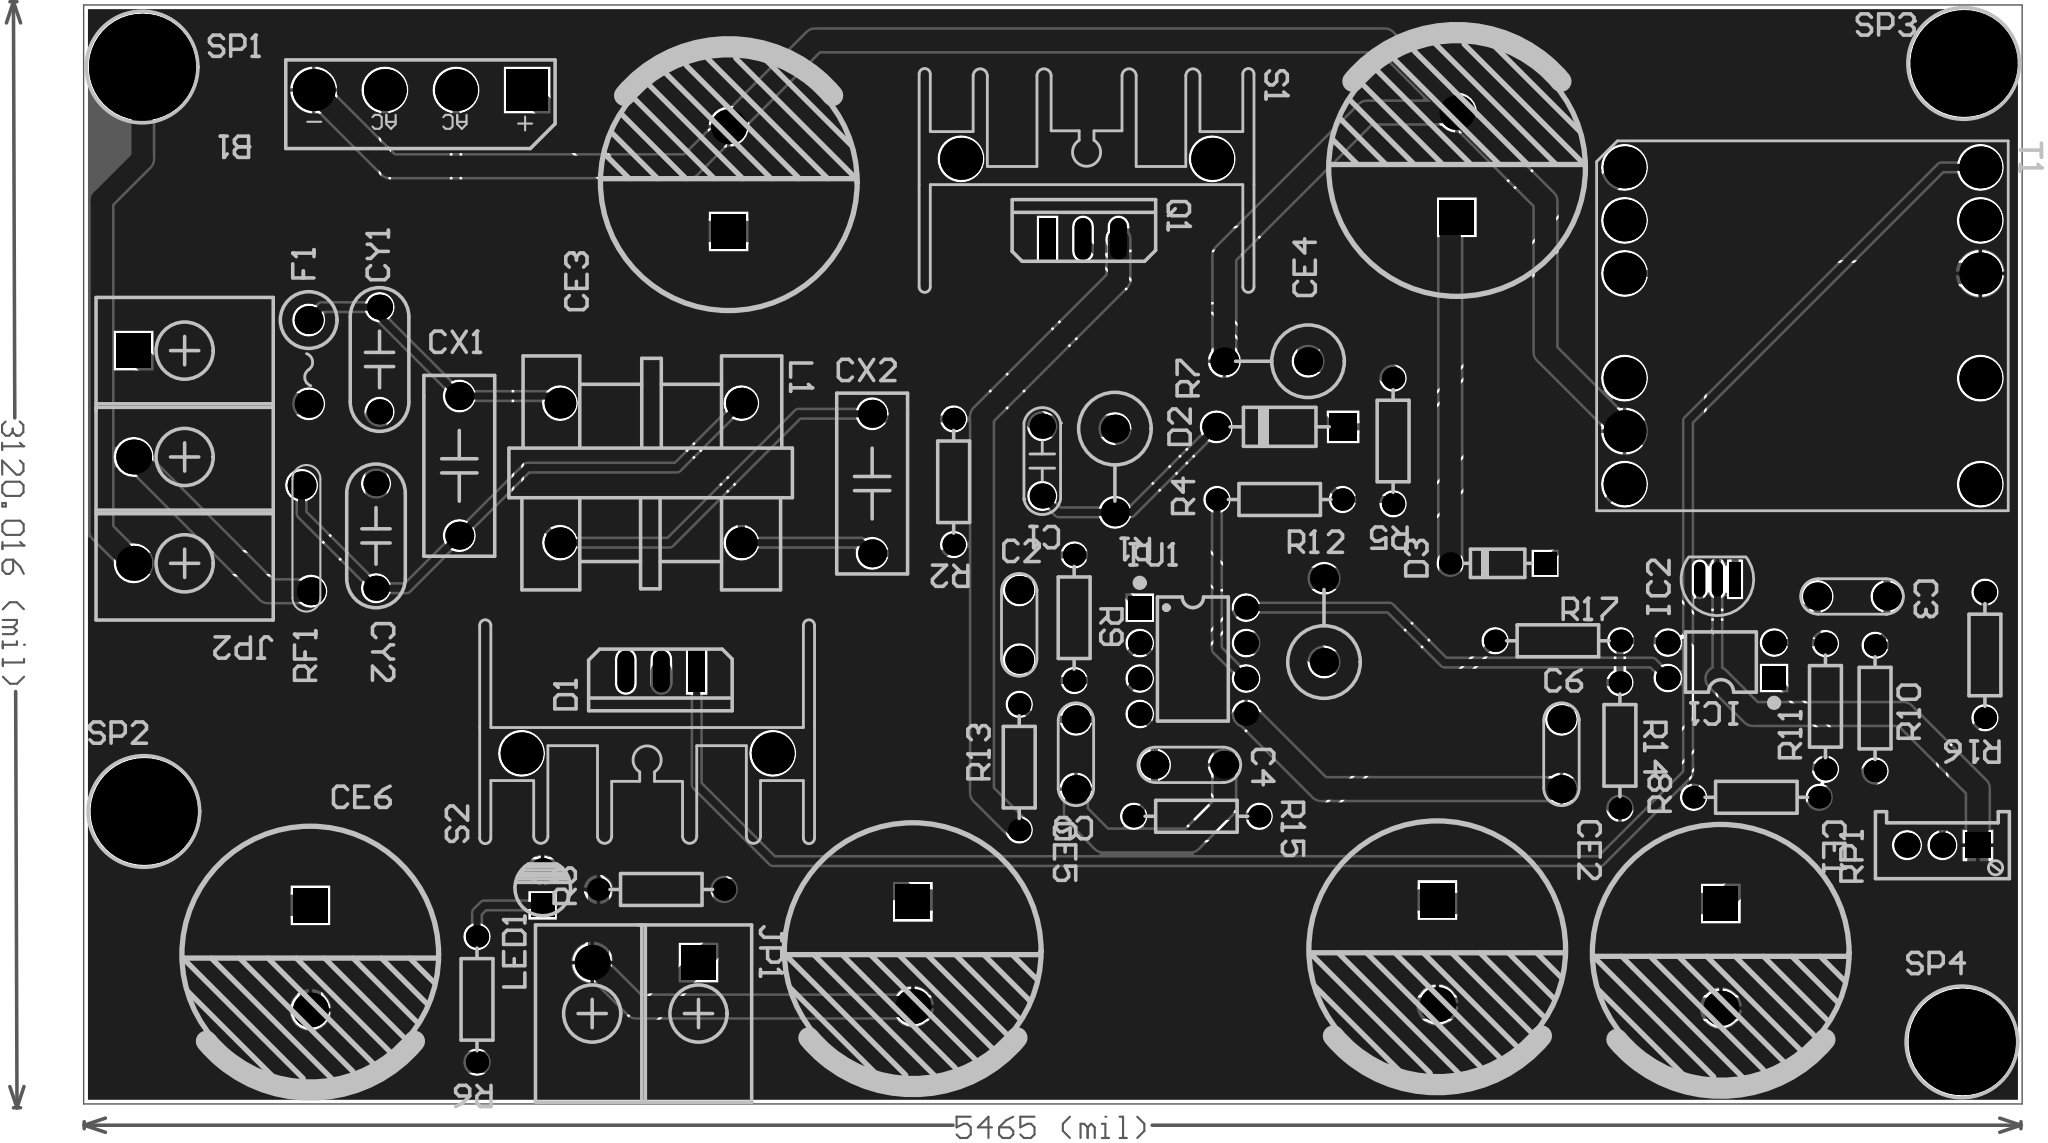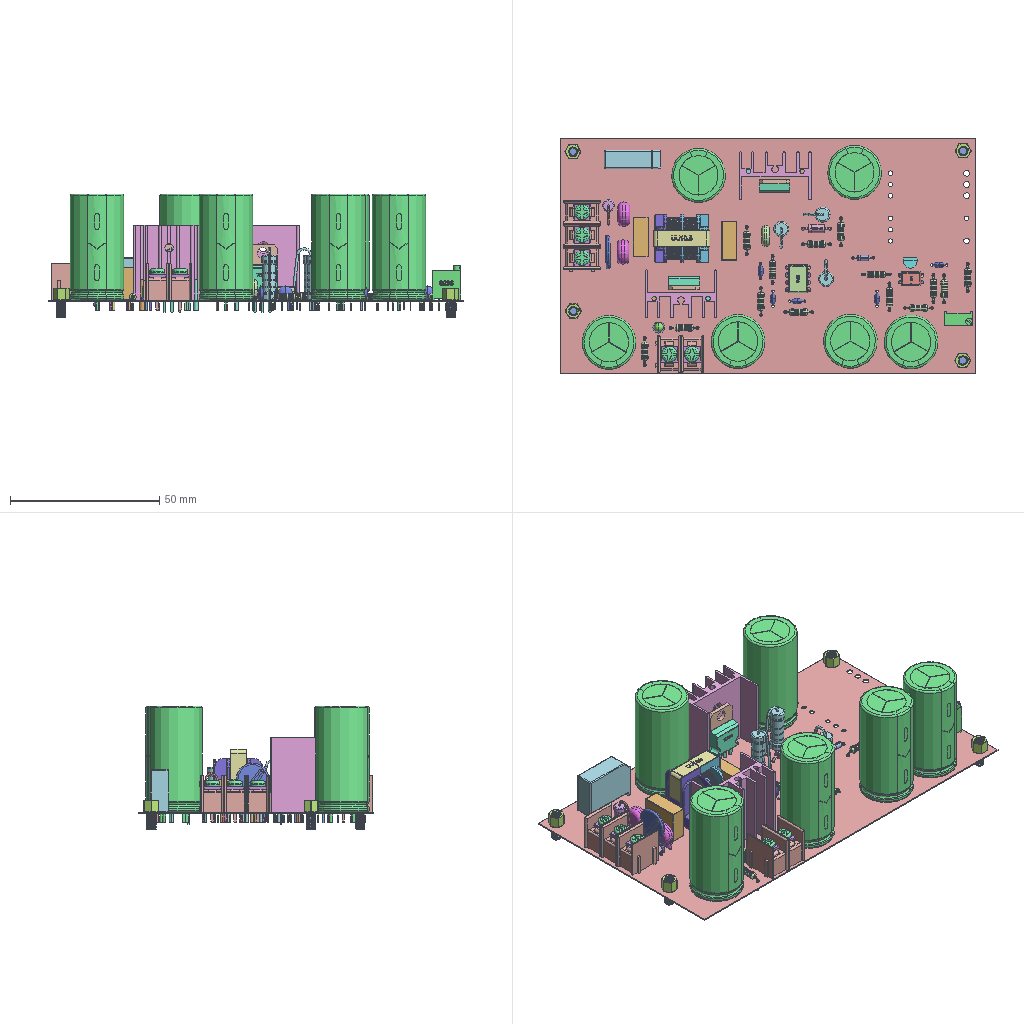Circuit board layout | Altium Designer | box 138.9 x 78.7 x 41.5 mm
Layer stack:
# Altium Designer layer stack of  (unit mm; dielectric type: 0 none, 1 core, 2 prepreg, 3 surface material)
index,name,kind,layer,copper_thickness_mm,dielectric_type,dielectric_thickness_mm,dielectric_material,dielectric_constant
0,Top Paste,other,,,,,,
1,Top Overlay,other,,,,,,
2,Top Solder,dielectric,,,3,0.0102,Solder Resist,3.5
3,Top Layer,copper,Top Layer,0.0356,,,,
4,Dielectric 1,dielectric,,,0,0.32,FR-4,4.8
5,Bottom Layer,copper,Bottom Layer,0.0356,,,,
6,Bottom Solder,dielectric,,,3,0.0102,Solder Resist,3.5
7,Bottom Overlay,other,,,,,,
8,Bottom Paste,other,,,,,,
# drill layer pairs: low layer,high layer
drill_pair,Top Layer,Bottom Layer
Part placement:
Designator,Comment,Layer,Footprint,Center-X(mm),Center-Y(mm),Rotation
T1,PQ2620,TopLayer,PQ2625+6PIN,145.161,99.06,270
SP4,M3 copper standoff,TopLayer,M3x4+6_N,156.591,47.752,0
SP3,M3 copper standoff,TopLayer,M3x4+6_N,156.718,117.856,0
SP2,M3 copper standoff,TopLayer,M3x4+6_N,26.289,64.262,0
SP1,M3 copper standoff,TopLayer,M3x4+6_N,26.162,117.602,0
S2,Heatsink,TopLayer,SRP16-24-25-P,62.357,68.427,180
S1,Heatsink,TopLayer,SRP16-24-25-P,93.853,111.024,360
RP1,500R,TopLayer,3296W,155.194,61.849,180
RF1,5D-11,TopLayer,TVR-10D,37.924,83.835,90
R17,1K/0.25W,TopLayer,RS_1/4W,127.635,76.492,360
R16,5.1K/0.25W,TopLayer,RS_1/4W,158.242,75.476,270
R15,8.87K/0.25W,TopLayer,RS_1/4W,101.727,63.919,360
R14,10K/0.25W,TopLayer,RS_1/4W,132.08,68.999,270
R13,1K/0.25W,TopLayer,RS_1/4W,89.027,67.437,90
R12,100K/2W,TopLayer,RS_2W-V6,110.871,77.968,90
R11,1K/0.25W,TopLayer,RS_1/4W,146.812,71.793,90
R10,20K/0.25W,TopLayer,RS_1/4W,150.368,71.666,90
R9,1K/0.25W,TopLayer,RS_1/4W,92.964,78.143,270
R8,270R/0.25W,TopLayer,RS_1/4W,141.859,65.278,180
R7,0.2Ω/2W,TopLayer,RS_2W-V6,106.728,96.52,180
R6,10K/0.25W,TopLayer,RS_1/4W,50.165,50.8,270
R5,10K/0.25W,TopLayer,RS_1/4W,115.824,90.805,270
R4,22Ω/0.25W,TopLayer,RS_1/4W,107.696,86.614,180
R3,1K/0.25W,TopLayer,RS_1/4W,63.373,58.674,180
R2,470K/0.25W,TopLayer,RS_1/4W,84.328,87.884,270
R1,100K/2W,TopLayer,RS_2W-V6,95.885,88.694,270
Q1,IPA90R1K2C3,TopLayer,TO220A,93.599,105.283,360
LED1,Green,TopLayer,LED_3MM-G,54.864,58.801,90
L1,20mH,TopLayer,UU10.5,62.611,88.519,360
JP2,HDR-1X3,TopLayer,KF7620-3P,25.56,89.662,270
JP1,HDR-1X2,TopLayer,KF7620-2P,62.23,53.434,180
IU1,UC3842,TopLayer,DIP8-300,101.473,75.057,360
IC2,TL431,TopLayer,TO92A,139.065,80.899,90
IC1,PC817,TopLayer,DIP4-300,139.319,75.095,180
F1,5x20/2A,TopLayer,FU_4x16_V,38.1,96.472,270
D3,1N4148,TopLayer,DO-35,123.317,82.042,180
D2,FR107,TopLayer,DO-41,107.696,91.821,180
D1,SBR20U100CT,TopLayer,TO220A,63.373,74.295,180
CY2,1nF/250VAC,TopLayer,CY_7.5*8*4,42.926,84.007,90
CY1,1nF/250VAC,TopLayer,CY_7.5*8*4,43.18,96.647,90
CX2,0.1uF/275V,TopLayer,CX_10-13*11,78.486,87.757,90
CX1,0.1uF/275V,TopLayer,CX_10-13*11,48.895,89.027,90
CE6,470uF/35V,TopLayer,CAP_7.5*18*35.5,38.227,53.788,270
CE5,470uF/35V,TopLayer,CAP_7.5*18*35.5,81.407,54.035,270
CE4,100uF/35V,TopLayer,CAP_7.5*18*35.5,120.396,110.587,90
CE3,120uF/450V,TopLayer,CAP_7.5*18*35.5,68.199,109.571,90
CE2,470uF/35V,TopLayer,CAP_7.5*18*35.5,118.999,54.169,270
CE1,470uF/35V,TopLayer,CAP_7.5*18*35.5,139.319,53.915,270
C6,1nF/50V,TopLayer,CC_2*5,127.889,68.364,90
C5,470pF/50V,TopLayer,CC_2*5,93.091,68.364,270
C4,2.2nF/50V,TopLayer,CC_2*5,101.219,67.602,360
C3,100nF/50V,TopLayer,CC_2*5,148.717,79.667,360
C2,10nF/50V,TopLayer,CC_2*5,89.027,77.635,90
C1,330pF/1KV,TopLayer,CY_5*7*2.5,90.678,89.368,270
B1,KBL606,TopLayer,KBL,46.111,115.951,180
Pad and via stacks:
# Altium Designer via and pad stacks of  (unit mm). Each distinct definition once, with the count of objects using it.
# via: kind,start_layer,end_layer,hole_mm,diameter_mm,mode(0 simple;1 top-mid-bottom;2 full stack),diameter_per_layer,count,example_net
# pad: kind,layer,hole_mm,hole_type(0 round;1 square;2 slot),plating,top_size,top_shape(1 round;2 rect;3 octagon;9 rounded rect),mid_size,bottom_size,mode,footprint,size_per_layer,count,example
pad,Multi-Layer,1.7,0,unplated,3x3,1,3x3,3x3,0,SRP16-24-25-P,,4,S2.0
pad,Multi-Layer,0.9,0,plated,2x2,1,2x2,2x2,0,FU 4x16_V,,2,F1.1
pad,Multi-Layer,1.5,0,plated,3x3,1,3x3,3x3,0,PQ2625+6PIN,,7,T1.9
pad,Multi-Layer,2,0,plated,3x3,1,3x3,3x3,0,PQ2625+6PIN,,4,T1.12
pad,Multi-Layer,0.8,0,plated,1.8x1.8,1,1.8x1.8,1.8x1.8,0,CY 5*7*2.5,,2,C1.1
pad,Multi-Layer,0.9,0,plated,2x2,1,2x2,2x2,0,RS 2W-V6,,6,R1.1
pad,Multi-Layer,0.8,0,plated,1.8x1.8,1,1.8x1.8,1.8x1.8,0,CY 7.5*8*4,,4,CY1.1
pad,Multi-Layer,1.1,0,plated,1.2x3,2,1.2x3,1.2x3,0,TO220A,,2,D1.1
pad,Multi-Layer,1.1,0,plated,1.2x3,1,1.2x3,1.2x3,0,TO220A,,4,D1.3
pad,Multi-Layer,1.6,0,plated,3x3,2,3x3,3x3,0,KBL,,1,B1.DC+
pad,Multi-Layer,1.6,0,plated,3x3,1,3x3,3x3,0,KBL,,3,B1.AC2
pad,Multi-Layer,1.2,0,plated,2.2x2.2,1,2.2x2.2,2.2x2.2,0,UU10.5,,4,L1.1
pad,Multi-Layer,1.4,0,plated,2.5x2.5,1,2.5x2.5,2.5x2.5,0,CAP 7.5*18*35.5,,6,CE6.2
pad,Multi-Layer,1.4,0,plated,2.5x2.5,2,2.5x2.5,2.5x2.5,0,CAP 7.5*18*35.5,,6,CE6.1
pad,Multi-Layer,1,0,plated,2x2,1,2x2,2x2,0,CX 10-13*11,,4,CX1.1
pad,Multi-Layer,1,0,plated,1.6x1.6,1,1.6x1.6,1.6x1.6,0,RS 1/4W,,28,R3.1
pad,Multi-Layer,1,0,plated,2x2,1,2x2,2x2,0,DO-41,,1,D2.2
pad,Multi-Layer,1,0,plated,2x2,2,2x2,2x2,0,DO-41,,1,D2.1
pad,Multi-Layer,1.2,0,plated,2.5x2.5,2,2.5x2.5,2.5x2.5,0,KF7620-2P,,1,JP1.1
pad,Multi-Layer,1.2,0,plated,2.5x2.5,1,2.5x2.5,2.5x2.5,0,KF7620-2P,,1,JP1.2
pad,Multi-Layer,1,0,plated,2x2,1,2x2,2x2,0,TVR-10D,,2,RF1.1
pad,Multi-Layer,0.8,0,plated,1.6x1.6,1,1.6x1.6,1.6x1.6,0,DO-35,,1,D3.2
pad,Multi-Layer,0.8,0,plated,1.6x1.6,2,1.6x1.6,1.6x1.6,0,DO-35,,1,D3.1
pad,Multi-Layer,0.9,0,plated,1.7x1.7,1,1.7x1.7,1.7x1.7,0,LED 3MM-G,,1,LED1.2
pad,Multi-Layer,0.9,0,plated,1.7x1.7,2,1.7x1.7,1.7x1.7,0,LED 3MM-G,,1,LED1.1
pad,Multi-Layer,1.2,0,plated,2.5x2.5,2,2.5x2.5,2.5x2.5,0,KF7620-3P,,1,JP2.1
pad,Multi-Layer,1.2,0,plated,2.5x2.5,1,2.5x2.5,2.5x2.5,0,KF7620-3P,,2,JP2.2
pad,Multi-Layer,0.8,0,plated,2x2,1,2x2,2x2,0,CC 2*5,,10,C2.2
pad,Multi-Layer,3.175,0,plated,7.62x7.62,1,7.62x7.62,7.62x7.62,0,M3x4+6_N,,4,SP4.1
pad,Multi-Layer,1,0,plated,1.7x1.7,2,1.7x1.7,1.7x1.7,0,DIP4-300,,1,IC1.1
pad,Multi-Layer,1,0,plated,1.7x1.7,1,1.7x1.7,1.7x1.7,0,DIP4-300,,3,IC1.2
pad,Multi-Layer,1,0,plated,1.7x1.7,1,1.7x1.7,1.7x1.7,0,DIP8-300,,7,IU1.8
pad,Multi-Layer,1,0,plated,1.7x1.7,2,1.7x1.7,1.7x1.7,0,DIP8-300,,1,IU1.1
pad,Multi-Layer,0.8,0,plated,2.5x0.8,1,2.5x0.8,2.5x0.8,0,TO92A,,2,IC2.3
pad,Multi-Layer,0.8,0,plated,2.5x0.8,2,2.5x0.8,2.5x0.8,0,TO92A,,1,IC2.1
pad,Multi-Layer,0.7,0,plated,1.8x1.8,2,1.8x1.8,1.8x1.8,0,3296W,,1,RP1.1
pad,Multi-Layer,0.7,0,plated,1.8x1.8,1,1.8x1.8,1.8x1.8,0,3296W,,2,RP1.2
Copper pours:
name,layer,net,type(0 solid;1 hatched;2 none)
Top Layer-No Net,Top Layer,SGND,0
Top Layer-No Net,Bottom Layer,PGND,0
Design rules, without the lines most boards share:
# Altium Designer design rules of  (exported by Altium Designer, unit mm)
# columns: name | kind | enabled | priority | scope1 | scope2 | descriptor | typed fields (field=value)
SilkToSilkClearance | 55 | enabled | 1 | All | All | Silk to Silk (Clearance=0mil) (All),(All) |
SilkToSolderMaskClearance | 54 | enabled | 1 | IsPad | All | Silk To Solder Mask (Clearance=0mil) (IsPad),(All) |
MinimumSolderMaskSliver | 53 | enabled | 1 | All | All | Minimum Solder Mask Sliver (Gap=0mil) (All),(All) |
HoleToHoleClearance | 52 | enabled | 1 | All | All | Hole To Hole Clearance (Gap=10mil) (All),(All) | gap=0.254
DiffPairsRouting | 51 | enabled | 1 | All | All | Differential Pairs Uncoupled Length using the Gap Constraints (Min=10mil) (Max=10mil) (Prefered=10mil)  and Width Constraints (Min=15mil) (Max=15mil) (Prefered=15mil) (All) |
Height | 50 | enabled | 1 | All | All | Height Constraint (Min=0mil) (Max=10000mil) (Prefered=500mil) (All) | min_height=0 max_height=254
SolderMaskExpansion | 13 | enabled | 1 | All | All | Solder Mask Expansion (Expansion =4mil) (All) | expansion=0.1016
PasteMaskExpansion | 14 | enabled | 1 | All | All | Paste Mask Expansion (Expansion =0mil) (All) | expansion=0
RoutingVias | 11 | enabled | 1 | All | All | Routing Via (MinHoleWidth=28mil) (MaxHoleWidth=28mil) (PreferredHoleWidth=28mil) (MinWidth=50mil) (MaxWidth=50mil) (PreferedWidth=50mil) (All) | via_min_hole=0.7112 via_max_hole=0.7112 via_preferred_diameter=1.27 via_preferred_hole=0.7112
Width | 2 | enabled | 1 | All | All | Width Constraint (Min=10mil) (Max=100mil) (Preferred=10mil) (All) |
PolygonConnect | 20 | enabled | 1 | All | All | Polygon Connect Rule(Relief Connect )(Conductor Width=10mil) (Relief Angle=90 Angle) (Entries=4) (Air Gap Width=10mil) (All),(All) | connect_style(0=relief,1=direct,2=none)=0 relief_conductor_width=0.254 relief_entries=4
PlaneConnect | 6 | enabled | 1 | All | All | Power Plane Connect Rule(Relief Connect )(Expansion=20mil) (Conductor Width=10mil) (Air Gap=10mil) (Entries=4) (All) | relief_conductor_width=0.254 relief_entries=4 relief_expansion=0.508
Clearance | 0 | enabled | 1 | All | All | Clearance Constraint (Gap=7mil) (All),(All) | gap=0.1778
Classes set for this board:
# Altium Designer classes of  (member kind: 0 net, 1 component, 2 from-to, 3 pad, 4 layer, 5 differential pair, 6 design channel, 7 polygon, 8 structure, 9 xSignal)
# columns: class name | member kind | superclass | members
CFY01205V1.2 | 1 | no | B1; C1; C2; C3; C4; C5; C6; CE1; CE2; CE3; CE4; CE5; CE6; CX1; CX2; CY1; CY2; D1; D2; D3; F1; IC1; IC2; IU1; JP1; JP2; L1; LED1; Q1; R1; R2; R3; R4; R5; R6; R7; R8; R9; R10; R11; R12; R13; R14; R15; R16; R17; RF1; RP1; S1; S2; SP1; SP2; SP3; SP4; T1;